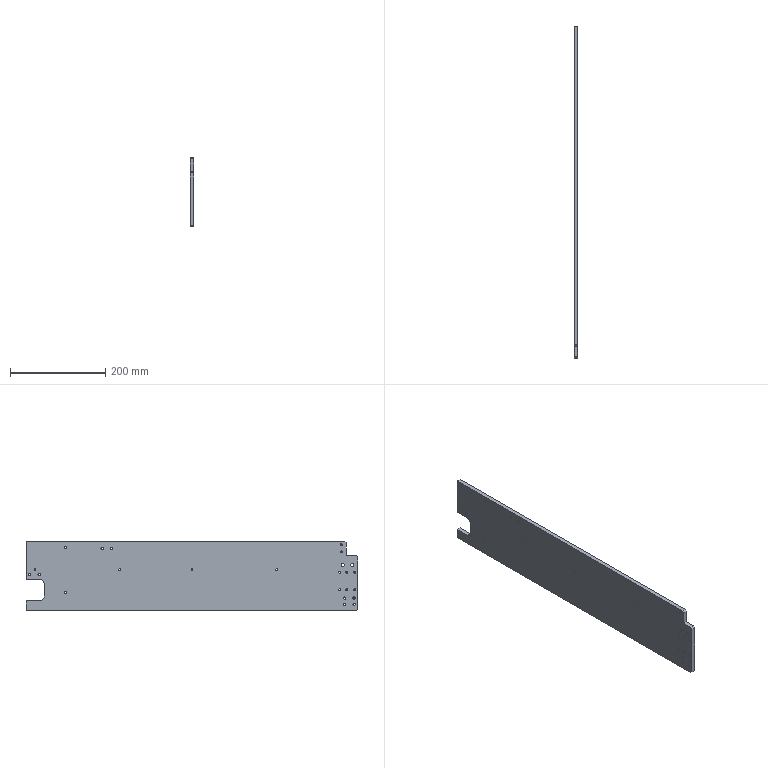Part | NX | features 5003_212_Side plate 2 | 1 solid | 43 faces | box 8 x 698 x 146 mm | volume 792240 mm3 | cylinder 26 | plane 15 | cone 2 | commonest cylinder face diameters 5 x10 4.2 x8 3.3 x4 6.6 x2 20 x2
STEP:
#1=CARTESIAN_POINT('',(-196.775,-63.6,-39.5));
#2=VERTEX_POINT('',#1);
#3=CARTESIAN_POINT('',(-196.775,-63.6,-42.));
#4=DIRECTION('',(1.,0.,0.));
#5=DIRECTION('',(0.,0.,1.));
#6=AXIS2_PLACEMENT_3D('',#3,#4,#5);
#7=CIRCLE('',#6,2.5);
#8=EDGE_CURVE('',#2,#2,#7,.T.);
#9=ORIENTED_EDGE('',*,*,#8,.T.);
#10=EDGE_LOOP('',(#9));
#11=FACE_BOUND('',#10,.T.);
#12=CARTESIAN_POINT('',(-196.775,-83.6,-39.5));
#13=VERTEX_POINT('',#12);
#14=CARTESIAN_POINT('',(-196.775,-83.6,-42.));
#15=DIRECTION('',(1.,0.,0.));
#16=DIRECTION('',(0.,0.,1.));
#17=AXIS2_PLACEMENT_3D('',#14,#15,#16);
#18=CIRCLE('',#17,2.5);
#19=EDGE_CURVE('',#13,#13,#18,.T.);
#20=ORIENTED_EDGE('',*,*,#19,.T.);
#21=EDGE_LOOP('',(#20));
#22=FACE_BOUND('',#21,.T.);
#23=CARTESIAN_POINT('',(-196.775,77.6,-88.15));
#24=VERTEX_POINT('',#23);
#25=CARTESIAN_POINT('',(-196.775,77.6,-86.5));
#26=DIRECTION('',(-1.,0.,0.));
#27=DIRECTION('',(0.,0.,-1.));
#28=AXIS2_PLACEMENT_3D('',#25,#26,#27);
#29=CIRCLE('',#28,1.65);
#30=EDGE_CURVE('',#24,#24,#29,.T.);
#31=ORIENTED_EDGE('',*,*,#30,.F.);
#32=EDGE_LOOP('',(#31));
#33=FACE_BOUND('',#32,.T.);
#34=CARTESIAN_POINT('',(-196.775,-100.2,-88.15));
#35=VERTEX_POINT('',#34);
#36=CARTESIAN_POINT('',(-196.775,-100.2,-86.5));
#37=DIRECTION('',(-1.,0.,0.));
#38=DIRECTION('',(0.,0.,-1.));
#39=AXIS2_PLACEMENT_3D('',#36,#37,#38);
#40=CIRCLE('',#39,1.65);
#41=EDGE_CURVE('',#35,#35,#40,.T.);
#42=ORIENTED_EDGE('',*,*,#41,.F.);
#43=EDGE_LOOP('',(#42));
#44=FACE_BOUND('',#43,.T.);
#45=CARTESIAN_POINT('',(-196.775,-430.4,-88.15));
#46=VERTEX_POINT('',#45);
#47=CARTESIAN_POINT('',(-196.775,-430.4,-86.5));
#48=DIRECTION('',(-1.,0.,0.));
#49=DIRECTION('',(0.,0.,-1.));
#50=AXIS2_PLACEMENT_3D('',#47,#48,#49);
#51=CIRCLE('',#50,1.65);
#52=EDGE_CURVE('',#46,#46,#51,.T.);
#53=ORIENTED_EDGE('',*,*,#52,.F.);
#54=EDGE_LOOP('',(#53));
#55=FACE_BOUND('',#54,.T.);
#56=CARTESIAN_POINT('',(-196.775,88.9,-99.58));
#57=VERTEX_POINT('',#56);
#58=CARTESIAN_POINT('',(-196.775,88.9,-97.08));
#59=DIRECTION('',(-1.,0.,0.));
#60=DIRECTION('',(0.,0.,-1.));
#61=AXIS2_PLACEMENT_3D('',#58,#59,#60);
#62=CIRCLE('',#61,2.5);
#63=EDGE_CURVE('',#57,#57,#62,.T.);
#64=ORIENTED_EDGE('',*,*,#63,.F.);
#65=EDGE_LOOP('',(#64));
#66=FACE_BOUND('',#65,.T.);
#67=CARTESIAN_POINT('',(-196.775,68.9,-99.58));
#68=VERTEX_POINT('',#67);
#69=CARTESIAN_POINT('',(-196.775,68.9,-97.08));
#70=DIRECTION('',(-1.,0.,0.));
#71=DIRECTION('',(0.,0.,-1.));
#72=AXIS2_PLACEMENT_3D('',#69,#70,#71);
#73=CIRCLE('',#72,2.5);
#74=EDGE_CURVE('',#68,#68,#73,.T.);
#75=ORIENTED_EDGE('',*,*,#74,.F.);
#76=EDGE_LOOP('',(#75));
#77=FACE_BOUND('',#76,.T.);
#78=CARTESIAN_POINT('',(-196.775,-573.6,-149.));
#79=VERTEX_POINT('',#78);
#80=CARTESIAN_POINT('',(-196.775,-573.6,-146.5));
#81=DIRECTION('',(-1.,0.,0.));
#82=DIRECTION('',(0.,0.,-1.));
#83=AXIS2_PLACEMENT_3D('',#80,#81,#82);
#84=CIRCLE('',#83,2.5);
#85=EDGE_CURVE('',#79,#79,#84,.T.);
#86=ORIENTED_EDGE('',*,*,#85,.F.);
#87=EDGE_LOOP('',(#86));
#88=FACE_BOUND('',#87,.T.);
#89=CARTESIAN_POINT('',(-196.775,-593.6,-149.));
#90=VERTEX_POINT('',#89);
#91=CARTESIAN_POINT('',(-196.775,-593.6,-146.5));
#92=DIRECTION('',(-1.,0.,0.));
#93=DIRECTION('',(0.,0.,-1.));
#94=AXIS2_PLACEMENT_3D('',#91,#92,#93);
#95=CIRCLE('',#94,2.5);
#96=EDGE_CURVE('',#90,#90,#95,.T.);
#97=ORIENTED_EDGE('',*,*,#96,.F.);
#98=EDGE_LOOP('',(#97));
#99=FACE_BOUND('',#98,.T.);
#100=CARTESIAN_POINT('',(-196.775,-593.6,-162.));
#101=VERTEX_POINT('',#100);
#102=CARTESIAN_POINT('',(-196.775,-593.6,-159.5));
#103=DIRECTION('',(-1.,0.,0.));
#104=DIRECTION('',(0.,0.,-1.));
#105=AXIS2_PLACEMENT_3D('',#102,#103,#104);
#106=CIRCLE('',#105,2.5);
#107=EDGE_CURVE('',#101,#101,#106,.T.);
#108=ORIENTED_EDGE('',*,*,#107,.F.);
#109=EDGE_LOOP('',(#108));
#110=FACE_BOUND('',#109,.T.);
#111=CARTESIAN_POINT('',(-196.775,13.9,-137.));
#112=VERTEX_POINT('',#111);
#113=CARTESIAN_POINT('',(-196.775,13.9,-134.5));
#114=DIRECTION('',(-1.,0.,0.));
#115=DIRECTION('',(0.,0.,-1.));
#116=AXIS2_PLACEMENT_3D('',#113,#114,#115);
#117=CIRCLE('',#116,2.5);
#118=EDGE_CURVE('',#112,#112,#117,.T.);
#119=ORIENTED_EDGE('',*,*,#118,.F.);
#120=EDGE_LOOP('',(#119));
#121=FACE_BOUND('',#120,.T.);
#122=CARTESIAN_POINT('',(-196.775,-566.6,-36.6));
#123=VERTEX_POINT('',#122);
#124=CARTESIAN_POINT('',(-196.775,-566.6,-34.5));
#125=DIRECTION('',(-1.,0.,0.));
#126=DIRECTION('',(0.,0.,-1.));
#127=AXIS2_PLACEMENT_3D('',#124,#125,#126);
#128=CIRCLE('',#127,2.1);
#129=EDGE_CURVE('',#123,#123,#128,.T.);
#130=ORIENTED_EDGE('',*,*,#129,.F.);
#131=EDGE_LOOP('',(#130));
#132=FACE_BOUND('',#131,.T.);
#133=CARTESIAN_POINT('',(-196.775,-566.6,-51.6));
#134=VERTEX_POINT('',#133);
#135=CARTESIAN_POINT('',(-196.775,-566.6,-49.5));
#136=DIRECTION('',(-1.,0.,0.));
#137=DIRECTION('',(0.,0.,-1.));
#138=AXIS2_PLACEMENT_3D('',#135,#136,#137);
#139=CIRCLE('',#138,2.1);
#140=EDGE_CURVE('',#134,#134,#139,.T.);
#141=ORIENTED_EDGE('',*,*,#140,.F.);
#142=EDGE_LOOP('',(#141));
#143=FACE_BOUND('',#142,.T.);
#144=CARTESIAN_POINT('',(-196.775,-563.1,-94.1));
#145=VERTEX_POINT('',#144);
#146=CARTESIAN_POINT('',(-196.775,-563.1,-92.));
#147=DIRECTION('',(-1.,0.,0.));
#148=DIRECTION('',(0.,0.,-1.));
#149=AXIS2_PLACEMENT_3D('',#146,#147,#148);
#150=CIRCLE('',#149,2.1);
#151=EDGE_CURVE('',#145,#145,#150,.T.);
#152=ORIENTED_EDGE('',*,*,#151,.F.);
#153=EDGE_LOOP('',(#152));
#154=FACE_BOUND('',#153,.T.);
#155=CARTESIAN_POINT('',(-196.775,-578.1,-94.1));
#156=VERTEX_POINT('',#155);
#157=CARTESIAN_POINT('',(-196.775,-578.1,-92.));
#158=DIRECTION('',(-1.,0.,0.));
#159=DIRECTION('',(0.,0.,-1.));
#160=AXIS2_PLACEMENT_3D('',#157,#158,#159);
#161=CIRCLE('',#160,2.1);
#162=EDGE_CURVE('',#156,#156,#161,.T.);
#163=ORIENTED_EDGE('',*,*,#162,.F.);
#164=EDGE_LOOP('',(#163));
#165=FACE_BOUND('',#164,.T.);
#166=CARTESIAN_POINT('',(-196.775,-595.1,-94.1));
#167=VERTEX_POINT('',#166);
#168=CARTESIAN_POINT('',(-196.775,-595.1,-92.));
#169=DIRECTION('',(-1.,0.,0.));
#170=DIRECTION('',(0.,0.,-1.));
#171=AXIS2_PLACEMENT_3D('',#168,#169,#170);
#172=CIRCLE('',#171,2.1);
#173=EDGE_CURVE('',#167,#167,#172,.T.);
#174=ORIENTED_EDGE('',*,*,#173,.F.);
#175=EDGE_LOOP('',(#174));
#176=FACE_BOUND('',#175,.T.);
#177=CARTESIAN_POINT('',(-196.775,-595.1,-131.1));
#178=VERTEX_POINT('',#177);
#179=CARTESIAN_POINT('',(-196.775,-595.1,-129.));
#180=DIRECTION('',(-1.,0.,0.));
#181=DIRECTION('',(0.,0.,-1.));
#182=AXIS2_PLACEMENT_3D('',#179,#180,#181);
#183=CIRCLE('',#182,2.1);
#184=EDGE_CURVE('',#178,#178,#183,.T.);
#185=ORIENTED_EDGE('',*,*,#184,.F.);
#186=EDGE_LOOP('',(#185));
#187=FACE_BOUND('',#186,.T.);
#188=CARTESIAN_POINT('',(-196.775,-578.1,-131.1));
#189=VERTEX_POINT('',#188);
#190=CARTESIAN_POINT('',(-196.775,-578.1,-129.));
#191=DIRECTION('',(-1.,0.,0.));
#192=DIRECTION('',(0.,0.,-1.));
#193=AXIS2_PLACEMENT_3D('',#190,#191,#192);
#194=CIRCLE('',#193,2.1);
#195=EDGE_CURVE('',#189,#189,#194,.T.);
#196=ORIENTED_EDGE('',*,*,#195,.F.);
#197=EDGE_LOOP('',(#196));
#198=FACE_BOUND('',#197,.T.);
#199=CARTESIAN_POINT('',(-196.775,-563.1,-131.1));
#200=VERTEX_POINT('',#199);
#201=CARTESIAN_POINT('',(-196.775,-563.1,-129.));
#202=DIRECTION('',(-1.,0.,0.));
#203=DIRECTION('',(0.,0.,-1.));
#204=AXIS2_PLACEMENT_3D('',#201,#202,#203);
#205=CIRCLE('',#204,2.1);
#206=EDGE_CURVE('',#200,#200,#205,.T.);
#207=ORIENTED_EDGE('',*,*,#206,.F.);
#208=EDGE_LOOP('',(#207));
#209=FACE_BOUND('',#208,.T.);
#210=CARTESIAN_POINT('',(-196.775,-569.6,-73.7));
#211=VERTEX_POINT('',#210);
#212=CARTESIAN_POINT('',(-196.775,-569.6,-77.));
#213=DIRECTION('',(1.,0.,0.));
#214=DIRECTION('',(0.,0.,1.));
#215=AXIS2_PLACEMENT_3D('',#212,#213,#214);
#216=CIRCLE('',#215,3.3);
#217=EDGE_CURVE('',#211,#211,#216,.T.);
#218=ORIENTED_EDGE('',*,*,#217,.T.);
#219=EDGE_LOOP('',(#218));
#220=FACE_BOUND('',#219,.T.);
#221=CARTESIAN_POINT('',(-196.775,-589.6,-73.7));
#222=VERTEX_POINT('',#221);
#223=CARTESIAN_POINT('',(-196.775,-589.6,-77.));
#224=DIRECTION('',(1.,0.,0.));
#225=DIRECTION('',(0.,0.,1.));
#226=AXIS2_PLACEMENT_3D('',#223,#224,#225);
#227=CIRCLE('',#226,3.3);
#228=EDGE_CURVE('',#222,#222,#227,.T.);
#229=ORIENTED_EDGE('',*,*,#228,.T.);
#230=EDGE_LOOP('',(#229));
#231=FACE_BOUND('',#230,.T.);
#232=CARTESIAN_POINT('',(-196.775,96.4,-173.));
#233=VERTEX_POINT('',#232);
#234=CARTESIAN_POINT('',(-196.775,-598.6,-173.));
#235=VERTEX_POINT('',#234);
#236=CARTESIAN_POINT('',(-196.775,-601.6,-173.));
#237=DIRECTION('',(0.,-1.,0.));
#238=VECTOR('',#237,1000.);
#239=LINE('',#236,#238);
#240=EDGE_CURVE('',#233,#235,#239,.T.);
#241=ORIENTED_EDGE('',*,*,#240,.T.);
#242=CARTESIAN_POINT('',(-196.775,-601.6,-170.));
#243=VERTEX_POINT('',#242);
#244=CARTESIAN_POINT('',(-196.775,-601.6,-170.));
#245=DIRECTION('',(0.,0.7071,-0.7071));
#246=VECTOR('',#245,1000.);
#247=LINE('',#244,#246);
#248=EDGE_CURVE('',#235,#243,#247,.F.);
#249=ORIENTED_EDGE('',*,*,#248,.T.);
#250=CARTESIAN_POINT('',(-196.775,-601.6,-60.));
#251=VERTEX_POINT('',#250);
#252=CARTESIAN_POINT('',(-196.775,-601.6,-57.));
#253=DIRECTION('',(0.,0.,1.));
#254=VECTOR('',#253,1000.);
#255=LINE('',#252,#254);
#256=EDGE_CURVE('',#243,#251,#255,.T.);
#257=ORIENTED_EDGE('',*,*,#256,.T.);
#258=CARTESIAN_POINT('',(-196.775,-598.6,-57.));
#259=VERTEX_POINT('',#258);
#260=CARTESIAN_POINT('',(-196.775,-598.6,-57.));
#261=DIRECTION('',(0.,-0.7071,-0.7071));
#262=VECTOR('',#261,1000.);
#263=LINE('',#260,#262);
#264=EDGE_CURVE('',#251,#259,#263,.F.);
#265=ORIENTED_EDGE('',*,*,#264,.T.);
#266=CARTESIAN_POINT('',(-196.775,-576.6,-57.));
#267=VERTEX_POINT('',#266);
#268=CARTESIAN_POINT('',(-196.775,-576.6,-57.));
#269=DIRECTION('',(0.,1.,0.));
#270=VECTOR('',#269,1000.);
#271=LINE('',#268,#270);
#272=EDGE_CURVE('',#259,#267,#271,.T.);
#273=ORIENTED_EDGE('',*,*,#272,.T.);
#274=CARTESIAN_POINT('',(-196.775,-576.6,-30.));
#275=VERTEX_POINT('',#274);
#276=CARTESIAN_POINT('',(-196.775,-576.6,-27.));
#277=DIRECTION('',(0.,0.,1.));
#278=VECTOR('',#277,1000.);
#279=LINE('',#276,#278);
#280=EDGE_CURVE('',#267,#275,#279,.T.);
#281=ORIENTED_EDGE('',*,*,#280,.T.);
#282=CARTESIAN_POINT('',(-196.775,-573.6,-27.));
#283=VERTEX_POINT('',#282);
#284=CARTESIAN_POINT('',(-196.775,-573.6,-27.));
#285=DIRECTION('',(0.,-0.7071,-0.7071));
#286=VECTOR('',#285,1000.);
#287=LINE('',#284,#286);
#288=EDGE_CURVE('',#275,#283,#287,.F.);
#289=ORIENTED_EDGE('',*,*,#288,.T.);
#290=CARTESIAN_POINT('',(-196.775,96.4,-27.));
#291=VERTEX_POINT('',#290);
#292=CARTESIAN_POINT('',(-196.775,96.4,-27.));
#293=DIRECTION('',(0.,1.,0.));
#294=VECTOR('',#293,1000.);
#295=LINE('',#292,#294);
#296=EDGE_CURVE('',#283,#291,#295,.T.);
#297=ORIENTED_EDGE('',*,*,#296,.T.);
#298=CARTESIAN_POINT('',(-196.775,96.4,-107.));
#299=VERTEX_POINT('',#298);
#300=CARTESIAN_POINT('',(-196.775,96.4,-107.));
#301=DIRECTION('',(0.,0.,-1.));
#302=VECTOR('',#301,1000.);
#303=LINE('',#300,#302);
#304=EDGE_CURVE('',#291,#299,#303,.T.);
#305=ORIENTED_EDGE('',*,*,#304,.T.);
#306=CARTESIAN_POINT('',(-196.775,68.4,-107.));
#307=VERTEX_POINT('',#306);
#308=CARTESIAN_POINT('',(-196.775,58.4,-107.));
#309=DIRECTION('',(0.,-1.,0.));
#310=VECTOR('',#309,1000.);
#311=LINE('',#308,#310);
#312=EDGE_CURVE('',#299,#307,#311,.T.);
#313=ORIENTED_EDGE('',*,*,#312,.T.);
#314=CARTESIAN_POINT('',(-196.775,58.4,-117.));
#315=VERTEX_POINT('',#314);
#316=CARTESIAN_POINT('',(-196.775,68.4,-117.));
#317=DIRECTION('',(1.,0.,0.));
#318=DIRECTION('',(0.,0.,1.));
#319=AXIS2_PLACEMENT_3D('',#316,#317,#318);
#320=CIRCLE('',#319,10.);
#321=EDGE_CURVE('',#307,#315,#320,.T.);
#322=ORIENTED_EDGE('',*,*,#321,.T.);
#323=CARTESIAN_POINT('',(-196.775,58.4,-142.));
#324=VERTEX_POINT('',#323);
#325=CARTESIAN_POINT('',(-196.775,58.4,-152.));
#326=DIRECTION('',(0.,0.,-1.));
#327=VECTOR('',#326,1000.);
#328=LINE('',#325,#327);
#329=EDGE_CURVE('',#315,#324,#328,.T.);
#330=ORIENTED_EDGE('',*,*,#329,.T.);
#331=CARTESIAN_POINT('',(-196.775,68.4,-152.));
#332=VERTEX_POINT('',#331);
#333=CARTESIAN_POINT('',(-196.775,68.4,-142.));
#334=DIRECTION('',(1.,0.,0.));
#335=DIRECTION('',(0.,0.,1.));
#336=AXIS2_PLACEMENT_3D('',#333,#334,#335);
#337=CIRCLE('',#336,10.);
#338=EDGE_CURVE('',#324,#332,#337,.T.);
#339=ORIENTED_EDGE('',*,*,#338,.T.);
#340=CARTESIAN_POINT('',(-196.775,96.4,-152.));
#341=VERTEX_POINT('',#340);
#342=CARTESIAN_POINT('',(-196.775,96.4,-152.));
#343=DIRECTION('',(0.,1.,0.));
#344=VECTOR('',#343,1000.);
#345=LINE('',#342,#344);
#346=EDGE_CURVE('',#332,#341,#345,.T.);
#347=ORIENTED_EDGE('',*,*,#346,.T.);
#348=CARTESIAN_POINT('',(-196.775,96.4,-173.));
#349=DIRECTION('',(0.,0.,-1.));
#350=VECTOR('',#349,1000.);
#351=LINE('',#348,#350);
#352=EDGE_CURVE('',#341,#233,#351,.T.);
#353=ORIENTED_EDGE('',*,*,#352,.T.);
#354=EDGE_LOOP('',(#241,#249,#257,#265,#273,#281,#289,#297,#305,#313,#322,#330,#339,#347,#353));
#355=FACE_BOUND('',#354,.T.);
#356=CARTESIAN_POINT('',(-196.775,13.9,-42.));
#357=VERTEX_POINT('',#356);
#358=CARTESIAN_POINT('',(-196.775,13.9,-39.5));
#359=DIRECTION('',(-1.,0.,0.));
#360=DIRECTION('',(0.,0.,-1.));
#361=AXIS2_PLACEMENT_3D('',#358,#359,#360);
#362=CIRCLE('',#361,2.5);
#363=EDGE_CURVE('',#357,#357,#362,.T.);
#364=ORIENTED_EDGE('',*,*,#363,.F.);
#365=EDGE_LOOP('',(#364));
#366=FACE_BOUND('',#365,.T.);
#367=CARTESIAN_POINT('',(-196.775,-573.6,-162.));
#368=VERTEX_POINT('',#367);
#369=CARTESIAN_POINT('',(-196.775,-573.6,-159.5));
#370=DIRECTION('',(-1.,0.,0.));
#371=DIRECTION('',(0.,0.,-1.));
#372=AXIS2_PLACEMENT_3D('',#369,#370,#371);
#373=CIRCLE('',#372,2.5);
#374=EDGE_CURVE('',#368,#368,#373,.T.);
#375=ORIENTED_EDGE('',*,*,#374,.F.);
#376=EDGE_LOOP('',(#375));
#377=FACE_BOUND('',#376,.T.);
#378=CARTESIAN_POINT('',(-196.775,-252.6,-88.15));
#379=VERTEX_POINT('',#378);
#380=CARTESIAN_POINT('',(-196.775,-252.6,-86.5));
#381=DIRECTION('',(-1.,0.,0.));
#382=DIRECTION('',(0.,0.,-1.));
#383=AXIS2_PLACEMENT_3D('',#380,#381,#382);
#384=CIRCLE('',#383,1.65);
#385=EDGE_CURVE('',#379,#379,#384,.T.);
#386=ORIENTED_EDGE('',*,*,#385,.F.);
#387=EDGE_LOOP('',(#386));
#388=FACE_BOUND('',#387,.T.);
#389=CARTESIAN_POINT('',(-196.775,96.4,-27.));
#390=DIRECTION('',(1.,0.,0.));
#391=DIRECTION('',(0.,0.,1.));
#392=AXIS2_PLACEMENT_3D('',#389,#390,#391);
#393=PLANE('',#392);
#394=ADVANCED_FACE('',(#11,#22,#33,#44,#55,#66,#77,#88,#99,#110,#121,#132,#143,#154,#165,#176,#187,#198,#209,#220,#231,#355,#366,#377,#388),#393,.F.);
#395=CARTESIAN_POINT('',(-188.775,96.4,-27.));
#396=VERTEX_POINT('',#395);
#397=CARTESIAN_POINT('',(-188.775,96.4,-107.));
#398=VERTEX_POINT('',#397);
#399=CARTESIAN_POINT('',(-188.775,96.4,-107.));
#400=DIRECTION('',(0.,0.,-1.));
#401=VECTOR('',#400,1000.);
#402=LINE('',#399,#401);
#403=EDGE_CURVE('',#396,#398,#402,.T.);
#404=ORIENTED_EDGE('',*,*,#403,.T.);
#405=CARTESIAN_POINT('',(-196.775,96.4,-107.));
#406=DIRECTION('',(1.,0.,0.));
#407=VECTOR('',#406,1000.);
#408=LINE('',#405,#407);
#409=EDGE_CURVE('',#299,#398,#408,.T.);
#410=ORIENTED_EDGE('',*,*,#409,.F.);
#411=ORIENTED_EDGE('',*,*,#304,.F.);
#412=CARTESIAN_POINT('',(-196.775,96.4,-27.));
#413=DIRECTION('',(1.,0.,0.));
#414=VECTOR('',#413,1000.);
#415=LINE('',#412,#414);
#416=EDGE_CURVE('',#291,#396,#415,.T.);
#417=ORIENTED_EDGE('',*,*,#416,.T.);
#418=EDGE_LOOP('',(#404,#410,#411,#417));
#419=FACE_BOUND('',#418,.T.);
#420=CARTESIAN_POINT('',(-196.775,96.4,-107.));
#421=DIRECTION('',(0.,-1.,0.));
#422=DIRECTION('',(0.,0.,1.));
#423=AXIS2_PLACEMENT_3D('',#420,#421,#422);
#424=PLANE('',#423);
#425=ADVANCED_FACE('',(#419),#424,.F.);
#426=CARTESIAN_POINT('',(-188.775,68.4,-107.));
#427=VERTEX_POINT('',#426);
#428=CARTESIAN_POINT('',(-188.775,58.4,-107.));
#429=DIRECTION('',(0.,-1.,0.));
#430=VECTOR('',#429,1000.);
#431=LINE('',#428,#430);
#432=EDGE_CURVE('',#398,#427,#431,.T.);
#433=ORIENTED_EDGE('',*,*,#432,.T.);
#434=CARTESIAN_POINT('',(-196.775,68.4,-107.));
#435=DIRECTION('',(1.,0.,0.));
#436=VECTOR('',#435,1000.);
#437=LINE('',#434,#436);
#438=EDGE_CURVE('',#427,#307,#437,.F.);
#439=ORIENTED_EDGE('',*,*,#438,.T.);
#440=ORIENTED_EDGE('',*,*,#312,.F.);
#441=ORIENTED_EDGE('',*,*,#409,.T.);
#442=EDGE_LOOP('',(#433,#439,#440,#441));
#443=FACE_BOUND('',#442,.T.);
#444=CARTESIAN_POINT('',(-196.775,58.4,-107.));
#445=DIRECTION('',(0.,0.,1.));
#446=DIRECTION('',(0.,1.,0.));
#447=AXIS2_PLACEMENT_3D('',#444,#445,#446);
#448=PLANE('',#447);
#449=ADVANCED_FACE('',(#443),#448,.F.);
#450=CARTESIAN_POINT('',(-188.775,58.4,-117.));
#451=VERTEX_POINT('',#450);
#452=CARTESIAN_POINT('',(-188.775,58.4,-142.));
#453=VERTEX_POINT('',#452);
#454=CARTESIAN_POINT('',(-188.775,58.4,-152.));
#455=DIRECTION('',(0.,0.,-1.));
#456=VECTOR('',#455,1000.);
#457=LINE('',#454,#456);
#458=EDGE_CURVE('',#451,#453,#457,.T.);
#459=ORIENTED_EDGE('',*,*,#458,.T.);
#460=CARTESIAN_POINT('',(-196.775,58.4,-142.));
#461=DIRECTION('',(1.,0.,0.));
#462=VECTOR('',#461,1000.);
#463=LINE('',#460,#462);
#464=EDGE_CURVE('',#453,#324,#463,.F.);
#465=ORIENTED_EDGE('',*,*,#464,.T.);
#466=ORIENTED_EDGE('',*,*,#329,.F.);
#467=CARTESIAN_POINT('',(-188.775,58.4,-117.));
#468=DIRECTION('',(1.,0.,0.));
#469=VECTOR('',#468,1000.);
#470=LINE('',#467,#469);
#471=EDGE_CURVE('',#315,#451,#470,.T.);
#472=ORIENTED_EDGE('',*,*,#471,.T.);
#473=EDGE_LOOP('',(#459,#465,#466,#472));
#474=FACE_BOUND('',#473,.T.);
#475=CARTESIAN_POINT('',(-196.775,58.4,-152.));
#476=DIRECTION('',(0.,-1.,0.));
#477=DIRECTION('',(0.,0.,1.));
#478=AXIS2_PLACEMENT_3D('',#475,#476,#477);
#479=PLANE('',#478);
#480=ADVANCED_FACE('',(#474),#479,.F.);
#481=ORIENTED_EDGE('',*,*,#346,.F.);
#482=CARTESIAN_POINT('',(-188.775,68.4,-152.));
#483=VERTEX_POINT('',#482);
#484=CARTESIAN_POINT('',(-188.775,68.4,-152.));
#485=DIRECTION('',(1.,0.,0.));
#486=VECTOR('',#485,1000.);
#487=LINE('',#484,#486);
#488=EDGE_CURVE('',#332,#483,#487,.T.);
#489=ORIENTED_EDGE('',*,*,#488,.T.);
#490=CARTESIAN_POINT('',(-188.775,96.4,-152.));
#491=VERTEX_POINT('',#490);
#492=CARTESIAN_POINT('',(-188.775,96.4,-152.));
#493=DIRECTION('',(0.,1.,0.));
#494=VECTOR('',#493,1000.);
#495=LINE('',#492,#494);
#496=EDGE_CURVE('',#483,#491,#495,.T.);
#497=ORIENTED_EDGE('',*,*,#496,.T.);
#498=CARTESIAN_POINT('',(-196.775,96.4,-152.));
#499=DIRECTION('',(1.,0.,0.));
#500=VECTOR('',#499,1000.);
#501=LINE('',#498,#500);
#502=EDGE_CURVE('',#341,#491,#501,.T.);
#503=ORIENTED_EDGE('',*,*,#502,.F.);
#504=EDGE_LOOP('',(#481,#489,#497,#503));
#505=FACE_BOUND('',#504,.T.);
#506=CARTESIAN_POINT('',(-196.775,96.4,-152.));
#507=DIRECTION('',(0.,0.,-1.));
#508=DIRECTION('',(0.,-1.,0.));
#509=AXIS2_PLACEMENT_3D('',#506,#507,#508);
#510=PLANE('',#509);
#511=ADVANCED_FACE('',(#505),#510,.F.);
#512=CARTESIAN_POINT('',(-188.775,96.4,-173.));
#513=VERTEX_POINT('',#512);
#514=CARTESIAN_POINT('',(-188.775,96.4,-173.));
#515=DIRECTION('',(0.,0.,-1.));
#516=VECTOR('',#515,1000.);
#517=LINE('',#514,#516);
#518=EDGE_CURVE('',#491,#513,#517,.T.);
#519=ORIENTED_EDGE('',*,*,#518,.T.);
#520=CARTESIAN_POINT('',(-196.775,96.4,-173.));
#521=DIRECTION('',(1.,0.,0.));
#522=VECTOR('',#521,1000.);
#523=LINE('',#520,#522);
#524=EDGE_CURVE('',#233,#513,#523,.T.);
#525=ORIENTED_EDGE('',*,*,#524,.F.);
#526=ORIENTED_EDGE('',*,*,#352,.F.);
#527=ORIENTED_EDGE('',*,*,#502,.T.);
#528=EDGE_LOOP('',(#519,#525,#526,#527));
#529=FACE_BOUND('',#528,.T.);
#530=CARTESIAN_POINT('',(-196.775,96.4,-173.));
#531=DIRECTION('',(0.,-1.,0.));
#532=DIRECTION('',(0.,0.,1.));
#533=AXIS2_PLACEMENT_3D('',#530,#531,#532);
#534=PLANE('',#533);
#535=ADVANCED_FACE('',(#529),#534,.F.);
#536=CARTESIAN_POINT('',(-188.775,-598.6,-173.));
#537=VERTEX_POINT('',#536);
#538=CARTESIAN_POINT('',(-188.775,-601.6,-173.));
#539=DIRECTION('',(0.,-1.,0.));
#540=VECTOR('',#539,1000.);
#541=LINE('',#538,#540);
#542=EDGE_CURVE('',#513,#537,#541,.T.);
#543=ORIENTED_EDGE('',*,*,#542,.T.);
#544=CARTESIAN_POINT('',(-196.775,-598.6,-173.));
#545=DIRECTION('',(-1.,0.,0.));
#546=VECTOR('',#545,1000.);
#547=LINE('',#544,#546);
#548=EDGE_CURVE('',#537,#235,#547,.T.);
#549=ORIENTED_EDGE('',*,*,#548,.T.);
#550=ORIENTED_EDGE('',*,*,#240,.F.);
#551=ORIENTED_EDGE('',*,*,#524,.T.);
#552=EDGE_LOOP('',(#543,#549,#550,#551));
#553=FACE_BOUND('',#552,.T.);
#554=CARTESIAN_POINT('',(-196.775,-601.6,-173.));
#555=DIRECTION('',(0.,0.,1.));
#556=DIRECTION('',(0.,1.,0.));
#557=AXIS2_PLACEMENT_3D('',#554,#555,#556);
#558=PLANE('',#557);
#559=ADVANCED_FACE('',(#553),#558,.F.);
#560=ORIENTED_EDGE('',*,*,#256,.F.);
#561=CARTESIAN_POINT('',(-188.775,-601.6,-170.));
#562=VERTEX_POINT('',#561);
#563=CARTESIAN_POINT('',(-196.775,-601.6,-170.));
#564=DIRECTION('',(1.,0.,0.));
#565=VECTOR('',#564,1000.);
#566=LINE('',#563,#565);
#567=EDGE_CURVE('',#243,#562,#566,.T.);
#568=ORIENTED_EDGE('',*,*,#567,.T.);
#569=CARTESIAN_POINT('',(-188.775,-601.6,-60.));
#570=VERTEX_POINT('',#569);
#571=CARTESIAN_POINT('',(-188.775,-601.6,-57.));
#572=DIRECTION('',(0.,0.,1.));
#573=VECTOR('',#572,1000.);
#574=LINE('',#571,#573);
#575=EDGE_CURVE('',#562,#570,#574,.T.);
#576=ORIENTED_EDGE('',*,*,#575,.T.);
#577=CARTESIAN_POINT('',(-196.775,-601.6,-60.));
#578=DIRECTION('',(-1.,0.,0.));
#579=VECTOR('',#578,1000.);
#580=LINE('',#577,#579);
#581=EDGE_CURVE('',#570,#251,#580,.T.);
#582=ORIENTED_EDGE('',*,*,#581,.T.);
#583=EDGE_LOOP('',(#560,#568,#576,#582));
#584=FACE_BOUND('',#583,.T.);
#585=CARTESIAN_POINT('',(-196.775,-601.6,-57.));
#586=DIRECTION('',(0.,1.,0.));
#587=DIRECTION('',(0.,0.,-1.));
#588=AXIS2_PLACEMENT_3D('',#585,#586,#587);
#589=PLANE('',#588);
#590=ADVANCED_FACE('',(#584),#589,.F.);
#591=ORIENTED_EDGE('',*,*,#272,.F.);
#592=CARTESIAN_POINT('',(-188.775,-598.6,-57.));
#593=VERTEX_POINT('',#592);
#594=CARTESIAN_POINT('',(-196.775,-598.6,-57.));
#595=DIRECTION('',(1.,0.,0.));
#596=VECTOR('',#595,1000.);
#597=LINE('',#594,#596);
#598=EDGE_CURVE('',#259,#593,#597,.T.);
#599=ORIENTED_EDGE('',*,*,#598,.T.);
#600=CARTESIAN_POINT('',(-188.775,-576.6,-57.));
#601=VERTEX_POINT('',#600);
#602=CARTESIAN_POINT('',(-188.775,-576.6,-57.));
#603=DIRECTION('',(0.,1.,0.));
#604=VECTOR('',#603,1000.);
#605=LINE('',#602,#604);
#606=EDGE_CURVE('',#593,#601,#605,.T.);
#607=ORIENTED_EDGE('',*,*,#606,.T.);
#608=CARTESIAN_POINT('',(-196.775,-576.6,-57.));
#609=DIRECTION('',(1.,0.,0.));
#610=VECTOR('',#609,1000.);
#611=LINE('',#608,#610);
#612=EDGE_CURVE('',#267,#601,#611,.T.);
#613=ORIENTED_EDGE('',*,*,#612,.F.);
#614=EDGE_LOOP('',(#591,#599,#607,#613));
#615=FACE_BOUND('',#614,.T.);
#616=CARTESIAN_POINT('',(-196.775,-576.6,-57.));
#617=DIRECTION('',(0.,0.,-1.));
#618=DIRECTION('',(0.,-1.,0.));
#619=AXIS2_PLACEMENT_3D('',#616,#617,#618);
#620=PLANE('',#619);
#621=ADVANCED_FACE('',(#615),#620,.F.);
#622=CARTESIAN_POINT('',(-188.775,-576.6,-30.));
#623=VERTEX_POINT('',#622);
#624=CARTESIAN_POINT('',(-188.775,-576.6,-27.));
#625=DIRECTION('',(0.,0.,1.));
#626=VECTOR('',#625,1000.);
#627=LINE('',#624,#626);
#628=EDGE_CURVE('',#601,#623,#627,.T.);
#629=ORIENTED_EDGE('',*,*,#628,.T.);
#630=CARTESIAN_POINT('',(-196.775,-576.6,-30.));
#631=DIRECTION('',(-1.,0.,0.));
#632=VECTOR('',#631,1000.);
#633=LINE('',#630,#632);
#634=EDGE_CURVE('',#623,#275,#633,.T.);
#635=ORIENTED_EDGE('',*,*,#634,.T.);
#636=ORIENTED_EDGE('',*,*,#280,.F.);
#637=ORIENTED_EDGE('',*,*,#612,.T.);
#638=EDGE_LOOP('',(#629,#635,#636,#637));
#639=FACE_BOUND('',#638,.T.);
#640=CARTESIAN_POINT('',(-196.775,-576.6,-27.));
#641=DIRECTION('',(0.,1.,0.));
#642=DIRECTION('',(0.,0.,-1.));
#643=AXIS2_PLACEMENT_3D('',#640,#641,#642);
#644=PLANE('',#643);
#645=ADVANCED_FACE('',(#639),#644,.F.);
#646=ORIENTED_EDGE('',*,*,#296,.F.);
#647=CARTESIAN_POINT('',(-188.775,-573.6,-27.));
#648=VERTEX_POINT('',#647);
#649=CARTESIAN_POINT('',(-196.775,-573.6,-27.));
#650=DIRECTION('',(1.,0.,0.));
#651=VECTOR('',#650,1000.);
#652=LINE('',#649,#651);
#653=EDGE_CURVE('',#283,#648,#652,.T.);
#654=ORIENTED_EDGE('',*,*,#653,.T.);
#655=CARTESIAN_POINT('',(-188.775,96.4,-27.));
#656=DIRECTION('',(0.,1.,0.));
#657=VECTOR('',#656,1000.);
#658=LINE('',#655,#657);
#659=EDGE_CURVE('',#648,#396,#658,.T.);
#660=ORIENTED_EDGE('',*,*,#659,.T.);
#661=ORIENTED_EDGE('',*,*,#416,.F.);
#662=EDGE_LOOP('',(#646,#654,#660,#661));
#663=FACE_BOUND('',#662,.T.);
#664=CARTESIAN_POINT('',(-196.775,96.4,-27.));
#665=DIRECTION('',(0.,0.,-1.));
#666=DIRECTION('',(0.,-1.,0.));
#667=AXIS2_PLACEMENT_3D('',#664,#665,#666);
#668=PLANE('',#667);
#669=ADVANCED_FACE('',(#663),#668,.F.);
#670=CARTESIAN_POINT('',(-188.775,-63.6,-39.5));
#671=VERTEX_POINT('',#670);
#672=CARTESIAN_POINT('',(-188.775,-63.6,-42.));
#673=DIRECTION('',(1.,0.,0.));
#674=DIRECTION('',(0.,0.,1.));
#675=AXIS2_PLACEMENT_3D('',#672,#673,#674);
#676=CIRCLE('',#675,2.5);
#677=EDGE_CURVE('',#671,#671,#676,.T.);
#678=ORIENTED_EDGE('',*,*,#677,.F.);
#679=EDGE_LOOP('',(#678));
#680=FACE_BOUND('',#679,.T.);
#681=CARTESIAN_POINT('',(-188.775,-83.6,-39.5));
#682=VERTEX_POINT('',#681);
#683=CARTESIAN_POINT('',(-188.775,-83.6,-42.));
#684=DIRECTION('',(1.,0.,0.));
#685=DIRECTION('',(0.,0.,1.));
#686=AXIS2_PLACEMENT_3D('',#683,#684,#685);
#687=CIRCLE('',#686,2.5);
#688=EDGE_CURVE('',#682,#682,#687,.T.);
#689=ORIENTED_EDGE('',*,*,#688,.F.);
#690=EDGE_LOOP('',(#689));
#691=FACE_BOUND('',#690,.T.);
#692=CARTESIAN_POINT('',(-188.775,77.6,-84.85));
#693=VERTEX_POINT('',#692);
#694=CARTESIAN_POINT('',(-188.775,77.6,-86.5));
#695=DIRECTION('',(1.,0.,0.));
#696=DIRECTION('',(0.,0.,1.));
#697=AXIS2_PLACEMENT_3D('',#694,#695,#696);
#698=CIRCLE('',#697,1.65);
#699=EDGE_CURVE('',#693,#693,#698,.T.);
#700=ORIENTED_EDGE('',*,*,#699,.F.);
#701=EDGE_LOOP('',(#700));
#702=FACE_BOUND('',#701,.T.);
#703=CARTESIAN_POINT('',(-188.775,-100.2,-84.85));
#704=VERTEX_POINT('',#703);
#705=CARTESIAN_POINT('',(-188.775,-100.2,-86.5));
#706=DIRECTION('',(1.,0.,0.));
#707=DIRECTION('',(0.,0.,1.));
#708=AXIS2_PLACEMENT_3D('',#705,#706,#707);
#709=CIRCLE('',#708,1.65);
#710=EDGE_CURVE('',#704,#704,#709,.T.);
#711=ORIENTED_EDGE('',*,*,#710,.F.);
#712=EDGE_LOOP('',(#711));
#713=FACE_BOUND('',#712,.T.);
#714=CARTESIAN_POINT('',(-188.775,-252.6,-84.85));
#715=VERTEX_POINT('',#714);
#716=CARTESIAN_POINT('',(-188.775,-252.6,-86.5));
#717=DIRECTION('',(1.,0.,0.));
#718=DIRECTION('',(0.,0.,1.));
#719=AXIS2_PLACEMENT_3D('',#716,#717,#718);
#720=CIRCLE('',#719,1.65);
#721=EDGE_CURVE('',#715,#715,#720,.T.);
#722=ORIENTED_EDGE('',*,*,#721,.F.);
#723=EDGE_LOOP('',(#722));
#724=FACE_BOUND('',#723,.T.);
#725=CARTESIAN_POINT('',(-188.775,-430.4,-84.85));
#726=VERTEX_POINT('',#725);
#727=CARTESIAN_POINT('',(-188.775,-430.4,-86.5));
#728=DIRECTION('',(1.,0.,0.));
#729=DIRECTION('',(0.,0.,1.));
#730=AXIS2_PLACEMENT_3D('',#727,#728,#729);
#731=CIRCLE('',#730,1.65);
#732=EDGE_CURVE('',#726,#726,#731,.T.);
#733=ORIENTED_EDGE('',*,*,#732,.F.);
#734=EDGE_LOOP('',(#733));
#735=FACE_BOUND('',#734,.T.);
#736=CARTESIAN_POINT('',(-188.775,88.9,-94.58));
#737=VERTEX_POINT('',#736);
#738=CARTESIAN_POINT('',(-188.775,88.9,-97.08));
#739=DIRECTION('',(1.,0.,0.));
#740=DIRECTION('',(0.,0.,1.));
#741=AXIS2_PLACEMENT_3D('',#738,#739,#740);
#742=CIRCLE('',#741,2.5);
#743=EDGE_CURVE('',#737,#737,#742,.T.);
#744=ORIENTED_EDGE('',*,*,#743,.F.);
#745=EDGE_LOOP('',(#744));
#746=FACE_BOUND('',#745,.T.);
#747=CARTESIAN_POINT('',(-188.775,68.9,-94.58));
#748=VERTEX_POINT('',#747);
#749=CARTESIAN_POINT('',(-188.775,68.9,-97.08));
#750=DIRECTION('',(1.,0.,0.));
#751=DIRECTION('',(0.,0.,1.));
#752=AXIS2_PLACEMENT_3D('',#749,#750,#751);
#753=CIRCLE('',#752,2.5);
#754=EDGE_CURVE('',#748,#748,#753,.T.);
#755=ORIENTED_EDGE('',*,*,#754,.F.);
#756=EDGE_LOOP('',(#755));
#757=FACE_BOUND('',#756,.T.);
#758=CARTESIAN_POINT('',(-188.775,-573.6,-144.));
#759=VERTEX_POINT('',#758);
#760=CARTESIAN_POINT('',(-188.775,-573.6,-146.5));
#761=DIRECTION('',(1.,0.,0.));
#762=DIRECTION('',(0.,0.,1.));
#763=AXIS2_PLACEMENT_3D('',#760,#761,#762);
#764=CIRCLE('',#763,2.5);
#765=EDGE_CURVE('',#759,#759,#764,.T.);
#766=ORIENTED_EDGE('',*,*,#765,.F.);
#767=EDGE_LOOP('',(#766));
#768=FACE_BOUND('',#767,.T.);
#769=CARTESIAN_POINT('',(-188.775,-593.6,-144.));
#770=VERTEX_POINT('',#769);
#771=CARTESIAN_POINT('',(-188.775,-593.6,-146.5));
#772=DIRECTION('',(1.,0.,0.));
#773=DIRECTION('',(0.,0.,1.));
#774=AXIS2_PLACEMENT_3D('',#771,#772,#773);
#775=CIRCLE('',#774,2.5);
#776=EDGE_CURVE('',#770,#770,#775,.T.);
#777=ORIENTED_EDGE('',*,*,#776,.F.);
#778=EDGE_LOOP('',(#777));
#779=FACE_BOUND('',#778,.T.);
#780=CARTESIAN_POINT('',(-188.775,-573.6,-157.));
#781=VERTEX_POINT('',#780);
#782=CARTESIAN_POINT('',(-188.775,-573.6,-159.5));
#783=DIRECTION('',(1.,0.,0.));
#784=DIRECTION('',(0.,0.,1.));
#785=AXIS2_PLACEMENT_3D('',#782,#783,#784);
#786=CIRCLE('',#785,2.5);
#787=EDGE_CURVE('',#781,#781,#786,.T.);
#788=ORIENTED_EDGE('',*,*,#787,.F.);
#789=EDGE_LOOP('',(#788));
#790=FACE_BOUND('',#789,.T.);
#791=CARTESIAN_POINT('',(-188.775,-593.6,-157.));
#792=VERTEX_POINT('',#791);
#793=CARTESIAN_POINT('',(-188.775,-593.6,-159.5));
#794=DIRECTION('',(1.,0.,0.));
#795=DIRECTION('',(0.,0.,1.));
#796=AXIS2_PLACEMENT_3D('',#793,#794,#795);
#797=CIRCLE('',#796,2.5);
#798=EDGE_CURVE('',#792,#792,#797,.T.);
#799=ORIENTED_EDGE('',*,*,#798,.F.);
#800=EDGE_LOOP('',(#799));
#801=FACE_BOUND('',#800,.T.);
#802=CARTESIAN_POINT('',(-188.775,13.9,-37.));
#803=VERTEX_POINT('',#802);
#804=CARTESIAN_POINT('',(-188.775,13.9,-39.5));
#805=DIRECTION('',(1.,0.,0.));
#806=DIRECTION('',(0.,0.,1.));
#807=AXIS2_PLACEMENT_3D('',#804,#805,#806);
#808=CIRCLE('',#807,2.5);
#809=EDGE_CURVE('',#803,#803,#808,.T.);
#810=ORIENTED_EDGE('',*,*,#809,.F.);
#811=EDGE_LOOP('',(#810));
#812=FACE_BOUND('',#811,.T.);
#813=CARTESIAN_POINT('',(-188.775,13.9,-132.));
#814=VERTEX_POINT('',#813);
#815=CARTESIAN_POINT('',(-188.775,13.9,-134.5));
#816=DIRECTION('',(1.,0.,0.));
#817=DIRECTION('',(0.,0.,1.));
#818=AXIS2_PLACEMENT_3D('',#815,#816,#817);
#819=CIRCLE('',#818,2.5);
#820=EDGE_CURVE('',#814,#814,#819,.T.);
#821=ORIENTED_EDGE('',*,*,#820,.F.);
#822=EDGE_LOOP('',(#821));
#823=FACE_BOUND('',#822,.T.);
#824=CARTESIAN_POINT('',(-188.775,-566.6,-32.4));
#825=VERTEX_POINT('',#824);
#826=CARTESIAN_POINT('',(-188.775,-566.6,-34.5));
#827=DIRECTION('',(1.,0.,0.));
#828=DIRECTION('',(0.,0.,1.));
#829=AXIS2_PLACEMENT_3D('',#826,#827,#828);
#830=CIRCLE('',#829,2.1);
#831=EDGE_CURVE('',#825,#825,#830,.T.);
#832=ORIENTED_EDGE('',*,*,#831,.F.);
#833=EDGE_LOOP('',(#832));
#834=FACE_BOUND('',#833,.T.);
#835=CARTESIAN_POINT('',(-188.775,-566.6,-47.4));
#836=VERTEX_POINT('',#835);
#837=CARTESIAN_POINT('',(-188.775,-566.6,-49.5));
#838=DIRECTION('',(1.,0.,0.));
#839=DIRECTION('',(0.,0.,1.));
#840=AXIS2_PLACEMENT_3D('',#837,#838,#839);
#841=CIRCLE('',#840,2.1);
#842=EDGE_CURVE('',#836,#836,#841,.T.);
#843=ORIENTED_EDGE('',*,*,#842,.F.);
#844=EDGE_LOOP('',(#843));
#845=FACE_BOUND('',#844,.T.);
#846=CARTESIAN_POINT('',(-188.775,-563.1,-89.9));
#847=VERTEX_POINT('',#846);
#848=CARTESIAN_POINT('',(-188.775,-563.1,-92.));
#849=DIRECTION('',(1.,0.,0.));
#850=DIRECTION('',(0.,0.,1.));
#851=AXIS2_PLACEMENT_3D('',#848,#849,#850);
#852=CIRCLE('',#851,2.1);
#853=EDGE_CURVE('',#847,#847,#852,.T.);
#854=ORIENTED_EDGE('',*,*,#853,.F.);
#855=EDGE_LOOP('',(#854));
#856=FACE_BOUND('',#855,.T.);
#857=CARTESIAN_POINT('',(-188.775,-578.1,-89.9));
#858=VERTEX_POINT('',#857);
#859=CARTESIAN_POINT('',(-188.775,-578.1,-92.));
#860=DIRECTION('',(1.,0.,0.));
#861=DIRECTION('',(0.,0.,1.));
#862=AXIS2_PLACEMENT_3D('',#859,#860,#861);
#863=CIRCLE('',#862,2.1);
#864=EDGE_CURVE('',#858,#858,#863,.T.);
#865=ORIENTED_EDGE('',*,*,#864,.F.);
#866=EDGE_LOOP('',(#865));
#867=FACE_BOUND('',#866,.T.);
#868=CARTESIAN_POINT('',(-188.775,-595.1,-89.9));
#869=VERTEX_POINT('',#868);
#870=CARTESIAN_POINT('',(-188.775,-595.1,-92.));
#871=DIRECTION('',(1.,0.,0.));
#872=DIRECTION('',(0.,0.,1.));
#873=AXIS2_PLACEMENT_3D('',#870,#871,#872);
#874=CIRCLE('',#873,2.1);
#875=EDGE_CURVE('',#869,#869,#874,.T.);
#876=ORIENTED_EDGE('',*,*,#875,.F.);
#877=EDGE_LOOP('',(#876));
#878=FACE_BOUND('',#877,.T.);
#879=CARTESIAN_POINT('',(-188.775,-595.1,-126.9));
#880=VERTEX_POINT('',#879);
#881=CARTESIAN_POINT('',(-188.775,-595.1,-129.));
#882=DIRECTION('',(1.,0.,0.));
#883=DIRECTION('',(0.,0.,1.));
#884=AXIS2_PLACEMENT_3D('',#881,#882,#883);
#885=CIRCLE('',#884,2.1);
#886=EDGE_CURVE('',#880,#880,#885,.T.);
#887=ORIENTED_EDGE('',*,*,#886,.F.);
#888=EDGE_LOOP('',(#887));
#889=FACE_BOUND('',#888,.T.);
#890=CARTESIAN_POINT('',(-188.775,-578.1,-126.9));
#891=VERTEX_POINT('',#890);
#892=CARTESIAN_POINT('',(-188.775,-578.1,-129.));
#893=DIRECTION('',(1.,0.,0.));
#894=DIRECTION('',(0.,0.,1.));
#895=AXIS2_PLACEMENT_3D('',#892,#893,#894);
#896=CIRCLE('',#895,2.1);
#897=EDGE_CURVE('',#891,#891,#896,.T.);
#898=ORIENTED_EDGE('',*,*,#897,.F.);
#899=EDGE_LOOP('',(#898));
#900=FACE_BOUND('',#899,.T.);
#901=CARTESIAN_POINT('',(-188.775,-563.1,-126.9));
#902=VERTEX_POINT('',#901);
#903=CARTESIAN_POINT('',(-188.775,-563.1,-129.));
#904=DIRECTION('',(1.,0.,0.));
#905=DIRECTION('',(0.,0.,1.));
#906=AXIS2_PLACEMENT_3D('',#903,#904,#905);
#907=CIRCLE('',#906,2.1);
#908=EDGE_CURVE('',#902,#902,#907,.T.);
#909=ORIENTED_EDGE('',*,*,#908,.F.);
#910=EDGE_LOOP('',(#909));
#911=FACE_BOUND('',#910,.T.);
#912=CARTESIAN_POINT('',(-188.775,-569.6,-70.4));
#913=VERTEX_POINT('',#912);
#914=CARTESIAN_POINT('',(-188.775,-569.6,-77.));
#915=DIRECTION('',(1.,0.,0.));
#916=DIRECTION('',(0.,0.,1.));
#917=AXIS2_PLACEMENT_3D('',#914,#915,#916);
#918=CIRCLE('',#917,6.6);
#919=EDGE_CURVE('',#913,#913,#918,.T.);
#920=ORIENTED_EDGE('',*,*,#919,.F.);
#921=EDGE_LOOP('',(#920));
#922=FACE_BOUND('',#921,.T.);
#923=CARTESIAN_POINT('',(-188.775,-589.6,-70.4));
#924=VERTEX_POINT('',#923);
#925=CARTESIAN_POINT('',(-188.775,-589.6,-77.));
#926=DIRECTION('',(1.,0.,0.));
#927=DIRECTION('',(0.,0.,1.));
#928=AXIS2_PLACEMENT_3D('',#925,#926,#927);
#929=CIRCLE('',#928,6.6);
#930=EDGE_CURVE('',#924,#924,#929,.T.);
#931=ORIENTED_EDGE('',*,*,#930,.F.);
#932=EDGE_LOOP('',(#931));
#933=FACE_BOUND('',#932,.T.);
#934=ORIENTED_EDGE('',*,*,#575,.F.);
#935=CARTESIAN_POINT('',(-188.775,-324.1,-447.5));
#936=DIRECTION('',(0.,-0.7071,0.7071));
#937=VECTOR('',#936,1000.);
#938=LINE('',#935,#937);
#939=EDGE_CURVE('',#562,#537,#938,.F.);
#940=ORIENTED_EDGE('',*,*,#939,.T.);
#941=ORIENTED_EDGE('',*,*,#542,.F.);
#942=ORIENTED_EDGE('',*,*,#518,.F.);
#943=ORIENTED_EDGE('',*,*,#496,.F.);
#944=CARTESIAN_POINT('',(-188.775,68.4,-142.));
#945=DIRECTION('',(1.,0.,0.));
#946=DIRECTION('',(0.,0.,1.));
#947=AXIS2_PLACEMENT_3D('',#944,#945,#946);
#948=CIRCLE('',#947,10.);
#949=EDGE_CURVE('',#483,#453,#948,.F.);
#950=ORIENTED_EDGE('',*,*,#949,.T.);
#951=ORIENTED_EDGE('',*,*,#458,.F.);
#952=CARTESIAN_POINT('',(-188.775,68.4,-117.));
#953=DIRECTION('',(1.,0.,0.));
#954=DIRECTION('',(0.,0.,1.));
#955=AXIS2_PLACEMENT_3D('',#952,#953,#954);
#956=CIRCLE('',#955,10.);
#957=EDGE_CURVE('',#451,#427,#956,.F.);
#958=ORIENTED_EDGE('',*,*,#957,.T.);
#959=ORIENTED_EDGE('',*,*,#432,.F.);
#960=ORIENTED_EDGE('',*,*,#403,.F.);
#961=ORIENTED_EDGE('',*,*,#659,.F.);
#962=CARTESIAN_POINT('',(-188.775,-238.6,308.));
#963=DIRECTION('',(0.,0.7071,0.7071));
#964=VECTOR('',#963,1000.);
#965=LINE('',#962,#964);
#966=EDGE_CURVE('',#648,#623,#965,.F.);
#967=ORIENTED_EDGE('',*,*,#966,.T.);
#968=ORIENTED_EDGE('',*,*,#628,.F.);
#969=ORIENTED_EDGE('',*,*,#606,.F.);
#970=CARTESIAN_POINT('',(-188.775,-236.1,305.5));
#971=DIRECTION('',(0.,0.7071,0.7071));
#972=VECTOR('',#971,1000.);
#973=LINE('',#970,#972);
#974=EDGE_CURVE('',#593,#570,#973,.F.);
#975=ORIENTED_EDGE('',*,*,#974,.T.);
#976=EDGE_LOOP('',(#934,#940,#941,#942,#943,#950,#951,#958,#959,#960,#961,#967,#968,#969,#975));
#977=FACE_BOUND('',#976,.T.);
#978=CARTESIAN_POINT('',(-188.775,96.4,-27.));
#979=DIRECTION('',(1.,0.,0.));
#980=DIRECTION('',(0.,0.,1.));
#981=AXIS2_PLACEMENT_3D('',#978,#979,#980);
#982=PLANE('',#981);
#983=ADVANCED_FACE('',(#680,#691,#702,#713,#724,#735,#746,#757,#768,#779,#790,#801,#812,#823,#834,#845,#856,#867,#878,#889,#900,#911,#922,#933,#977),#982,.T.);
#984=ORIENTED_EDGE('',*,*,#321,.F.);
#985=ORIENTED_EDGE('',*,*,#438,.F.);
#986=ORIENTED_EDGE('',*,*,#957,.F.);
#987=ORIENTED_EDGE('',*,*,#471,.F.);
#988=EDGE_LOOP('',(#984,#985,#986,#987));
#989=FACE_BOUND('',#988,.T.);
#990=CARTESIAN_POINT('',(-196.775,68.4,-117.));
#991=DIRECTION('',(-1.,0.,0.));
#992=DIRECTION('',(0.,0.,-1.));
#993=AXIS2_PLACEMENT_3D('',#990,#991,#992);
#994=CYLINDRICAL_SURFACE('',#993,10.);
#995=ADVANCED_FACE('',(#989),#994,.F.);
#996=ORIENTED_EDGE('',*,*,#338,.F.);
#997=ORIENTED_EDGE('',*,*,#464,.F.);
#998=ORIENTED_EDGE('',*,*,#949,.F.);
#999=ORIENTED_EDGE('',*,*,#488,.F.);
#1000=EDGE_LOOP('',(#996,#997,#998,#999));
#1001=FACE_BOUND('',#1000,.T.);
#1002=CARTESIAN_POINT('',(-196.775,68.4,-142.));
#1003=DIRECTION('',(-1.,0.,0.));
#1004=DIRECTION('',(0.,0.,-1.));
#1005=AXIS2_PLACEMENT_3D('',#1002,#1003,#1004);
#1006=CYLINDRICAL_SURFACE('',#1005,10.);
#1007=ADVANCED_FACE('',(#1001),#1006,.F.);
#1008=ORIENTED_EDGE('',*,*,#288,.F.);
#1009=ORIENTED_EDGE('',*,*,#634,.F.);
#1010=ORIENTED_EDGE('',*,*,#966,.F.);
#1011=ORIENTED_EDGE('',*,*,#653,.F.);
#1012=EDGE_LOOP('',(#1008,#1009,#1010,#1011));
#1013=FACE_BOUND('',#1012,.T.);
#1014=CARTESIAN_POINT('',(-196.775,-573.6,-27.));
#1015=DIRECTION('',(0.,0.7071,-0.7071));
#1016=DIRECTION('',(1.,0.,0.));
#1017=AXIS2_PLACEMENT_3D('',#1014,#1015,#1016);
#1018=PLANE('',#1017);
#1019=ADVANCED_FACE('',(#1013),#1018,.F.);
#1020=ORIENTED_EDGE('',*,*,#264,.F.);
#1021=ORIENTED_EDGE('',*,*,#581,.F.);
#1022=ORIENTED_EDGE('',*,*,#974,.F.);
#1023=ORIENTED_EDGE('',*,*,#598,.F.);
#1024=EDGE_LOOP('',(#1020,#1021,#1022,#1023));
#1025=FACE_BOUND('',#1024,.T.);
#1026=CARTESIAN_POINT('',(-196.775,-598.6,-57.));
#1027=DIRECTION('',(0.,0.7071,-0.7071));
#1028=DIRECTION('',(1.,0.,0.));
#1029=AXIS2_PLACEMENT_3D('',#1026,#1027,#1028);
#1030=PLANE('',#1029);
#1031=ADVANCED_FACE('',(#1025),#1030,.F.);
#1032=ORIENTED_EDGE('',*,*,#248,.F.);
#1033=ORIENTED_EDGE('',*,*,#548,.F.);
#1034=ORIENTED_EDGE('',*,*,#939,.F.);
#1035=ORIENTED_EDGE('',*,*,#567,.F.);
#1036=EDGE_LOOP('',(#1032,#1033,#1034,#1035));
#1037=FACE_BOUND('',#1036,.T.);
#1038=CARTESIAN_POINT('',(-196.775,-601.6,-170.));
#1039=DIRECTION('',(0.,0.7071,0.7071));
#1040=DIRECTION('',(1.,0.,0.));
#1041=AXIS2_PLACEMENT_3D('',#1038,#1039,#1040);
#1042=PLANE('',#1041);
#1043=ADVANCED_FACE('',(#1037),#1042,.F.);
#1044=ORIENTED_EDGE('',*,*,#228,.F.);
#1045=EDGE_LOOP('',(#1044));
#1046=FACE_BOUND('',#1045,.T.);
#1047=CARTESIAN_POINT('',(-192.075,-589.6,-73.7));
#1048=VERTEX_POINT('',#1047);
#1049=CARTESIAN_POINT('',(-192.075,-589.6,-77.));
#1050=DIRECTION('',(1.,0.,0.));
#1051=DIRECTION('',(0.,0.,1.));
#1052=AXIS2_PLACEMENT_3D('',#1049,#1050,#1051);
#1053=CIRCLE('',#1052,3.3);
#1054=EDGE_CURVE('',#1048,#1048,#1053,.T.);
#1055=ORIENTED_EDGE('',*,*,#1054,.T.);
#1056=EDGE_LOOP('',(#1055));
#1057=FACE_BOUND('',#1056,.T.);
#1058=CARTESIAN_POINT('',(-188.775,-589.6,-77.));
#1059=DIRECTION('',(1.,0.,0.));
#1060=DIRECTION('',(0.,0.,1.));
#1061=AXIS2_PLACEMENT_3D('',#1058,#1059,#1060);
#1062=CYLINDRICAL_SURFACE('',#1061,3.3);
#1063=ADVANCED_FACE('',(#1046,#1057),#1062,.F.);
#1064=ORIENTED_EDGE('',*,*,#1054,.F.);
#1065=EDGE_LOOP('',(#1064));
#1066=FACE_BOUND('',#1065,.T.);
#1067=ORIENTED_EDGE('',*,*,#930,.T.);
#1068=EDGE_LOOP('',(#1067));
#1069=FACE_BOUND('',#1068,.T.);
#1070=CARTESIAN_POINT('',(-188.775,-589.6,-77.));
#1071=DIRECTION('',(1.,0.,0.));
#1072=DIRECTION('',(0.,0.,1.));
#1073=AXIS2_PLACEMENT_3D('',#1070,#1071,#1072);
#1074=CONICAL_SURFACE('',#1073,6.6,0.7854);
#1075=ADVANCED_FACE('',(#1066,#1069),#1074,.F.);
#1076=ORIENTED_EDGE('',*,*,#217,.F.);
#1077=EDGE_LOOP('',(#1076));
#1078=FACE_BOUND('',#1077,.T.);
#1079=CARTESIAN_POINT('',(-192.075,-569.6,-73.7));
#1080=VERTEX_POINT('',#1079);
#1081=CARTESIAN_POINT('',(-192.075,-569.6,-77.));
#1082=DIRECTION('',(1.,0.,0.));
#1083=DIRECTION('',(0.,0.,1.));
#1084=AXIS2_PLACEMENT_3D('',#1081,#1082,#1083);
#1085=CIRCLE('',#1084,3.3);
#1086=EDGE_CURVE('',#1080,#1080,#1085,.T.);
#1087=ORIENTED_EDGE('',*,*,#1086,.T.);
#1088=EDGE_LOOP('',(#1087));
#1089=FACE_BOUND('',#1088,.T.);
#1090=CARTESIAN_POINT('',(-188.775,-569.6,-77.));
#1091=DIRECTION('',(1.,0.,0.));
#1092=DIRECTION('',(0.,0.,1.));
#1093=AXIS2_PLACEMENT_3D('',#1090,#1091,#1092);
#1094=CYLINDRICAL_SURFACE('',#1093,3.3);
#1095=ADVANCED_FACE('',(#1078,#1089),#1094,.F.);
#1096=ORIENTED_EDGE('',*,*,#1086,.F.);
#1097=EDGE_LOOP('',(#1096));
#1098=FACE_BOUND('',#1097,.T.);
#1099=ORIENTED_EDGE('',*,*,#919,.T.);
#1100=EDGE_LOOP('',(#1099));
#1101=FACE_BOUND('',#1100,.T.);
#1102=CARTESIAN_POINT('',(-188.775,-569.6,-77.));
#1103=DIRECTION('',(1.,0.,0.));
#1104=DIRECTION('',(0.,0.,1.));
#1105=AXIS2_PLACEMENT_3D('',#1102,#1103,#1104);
#1106=CONICAL_SURFACE('',#1105,6.6,0.7854);
#1107=ADVANCED_FACE('',(#1098,#1101),#1106,.F.);
#1108=ORIENTED_EDGE('',*,*,#908,.T.);
#1109=EDGE_LOOP('',(#1108));
#1110=FACE_BOUND('',#1109,.T.);
#1111=ORIENTED_EDGE('',*,*,#206,.T.);
#1112=EDGE_LOOP('',(#1111));
#1113=FACE_BOUND('',#1112,.T.);
#1114=CARTESIAN_POINT('',(-196.775,-563.1,-129.));
#1115=DIRECTION('',(-1.,0.,0.));
#1116=DIRECTION('',(0.,0.,-1.));
#1117=AXIS2_PLACEMENT_3D('',#1114,#1115,#1116);
#1118=CYLINDRICAL_SURFACE('',#1117,2.1);
#1119=ADVANCED_FACE('',(#1110,#1113),#1118,.F.);
#1120=ORIENTED_EDGE('',*,*,#897,.T.);
#1121=EDGE_LOOP('',(#1120));
#1122=FACE_BOUND('',#1121,.T.);
#1123=ORIENTED_EDGE('',*,*,#195,.T.);
#1124=EDGE_LOOP('',(#1123));
#1125=FACE_BOUND('',#1124,.T.);
#1126=CARTESIAN_POINT('',(-196.775,-578.1,-129.));
#1127=DIRECTION('',(-1.,0.,0.));
#1128=DIRECTION('',(0.,0.,-1.));
#1129=AXIS2_PLACEMENT_3D('',#1126,#1127,#1128);
#1130=CYLINDRICAL_SURFACE('',#1129,2.1);
#1131=ADVANCED_FACE('',(#1122,#1125),#1130,.F.);
#1132=ORIENTED_EDGE('',*,*,#886,.T.);
#1133=EDGE_LOOP('',(#1132));
#1134=FACE_BOUND('',#1133,.T.);
#1135=ORIENTED_EDGE('',*,*,#184,.T.);
#1136=EDGE_LOOP('',(#1135));
#1137=FACE_BOUND('',#1136,.T.);
#1138=CARTESIAN_POINT('',(-196.775,-595.1,-129.));
#1139=DIRECTION('',(-1.,0.,0.));
#1140=DIRECTION('',(0.,0.,-1.));
#1141=AXIS2_PLACEMENT_3D('',#1138,#1139,#1140);
#1142=CYLINDRICAL_SURFACE('',#1141,2.1);
#1143=ADVANCED_FACE('',(#1134,#1137),#1142,.F.);
#1144=ORIENTED_EDGE('',*,*,#875,.T.);
#1145=EDGE_LOOP('',(#1144));
#1146=FACE_BOUND('',#1145,.T.);
#1147=ORIENTED_EDGE('',*,*,#173,.T.);
#1148=EDGE_LOOP('',(#1147));
#1149=FACE_BOUND('',#1148,.T.);
#1150=CARTESIAN_POINT('',(-196.775,-595.1,-92.));
#1151=DIRECTION('',(-1.,0.,0.));
#1152=DIRECTION('',(0.,0.,-1.));
#1153=AXIS2_PLACEMENT_3D('',#1150,#1151,#1152);
#1154=CYLINDRICAL_SURFACE('',#1153,2.1);
#1155=ADVANCED_FACE('',(#1146,#1149),#1154,.F.);
#1156=ORIENTED_EDGE('',*,*,#864,.T.);
#1157=EDGE_LOOP('',(#1156));
#1158=FACE_BOUND('',#1157,.T.);
#1159=ORIENTED_EDGE('',*,*,#162,.T.);
#1160=EDGE_LOOP('',(#1159));
#1161=FACE_BOUND('',#1160,.T.);
#1162=CARTESIAN_POINT('',(-196.775,-578.1,-92.));
#1163=DIRECTION('',(-1.,0.,0.));
#1164=DIRECTION('',(0.,0.,-1.));
#1165=AXIS2_PLACEMENT_3D('',#1162,#1163,#1164);
#1166=CYLINDRICAL_SURFACE('',#1165,2.1);
#1167=ADVANCED_FACE('',(#1158,#1161),#1166,.F.);
#1168=ORIENTED_EDGE('',*,*,#853,.T.);
#1169=EDGE_LOOP('',(#1168));
#1170=FACE_BOUND('',#1169,.T.);
#1171=ORIENTED_EDGE('',*,*,#151,.T.);
#1172=EDGE_LOOP('',(#1171));
#1173=FACE_BOUND('',#1172,.T.);
#1174=CARTESIAN_POINT('',(-196.775,-563.1,-92.));
#1175=DIRECTION('',(-1.,0.,0.));
#1176=DIRECTION('',(0.,0.,-1.));
#1177=AXIS2_PLACEMENT_3D('',#1174,#1175,#1176);
#1178=CYLINDRICAL_SURFACE('',#1177,2.1);
#1179=ADVANCED_FACE('',(#1170,#1173),#1178,.F.);
#1180=ORIENTED_EDGE('',*,*,#842,.T.);
#1181=EDGE_LOOP('',(#1180));
#1182=FACE_BOUND('',#1181,.T.);
#1183=ORIENTED_EDGE('',*,*,#140,.T.);
#1184=EDGE_LOOP('',(#1183));
#1185=FACE_BOUND('',#1184,.T.);
#1186=CARTESIAN_POINT('',(-196.775,-566.6,-49.5));
#1187=DIRECTION('',(-1.,0.,0.));
#1188=DIRECTION('',(0.,0.,-1.));
#1189=AXIS2_PLACEMENT_3D('',#1186,#1187,#1188);
#1190=CYLINDRICAL_SURFACE('',#1189,2.1);
#1191=ADVANCED_FACE('',(#1182,#1185),#1190,.F.);
#1192=ORIENTED_EDGE('',*,*,#831,.T.);
#1193=EDGE_LOOP('',(#1192));
#1194=FACE_BOUND('',#1193,.T.);
#1195=ORIENTED_EDGE('',*,*,#129,.T.);
#1196=EDGE_LOOP('',(#1195));
#1197=FACE_BOUND('',#1196,.T.);
#1198=CARTESIAN_POINT('',(-196.775,-566.6,-34.5));
#1199=DIRECTION('',(-1.,0.,0.));
#1200=DIRECTION('',(0.,0.,-1.));
#1201=AXIS2_PLACEMENT_3D('',#1198,#1199,#1200);
#1202=CYLINDRICAL_SURFACE('',#1201,2.1);
#1203=ADVANCED_FACE('',(#1194,#1197),#1202,.F.);
#1204=ORIENTED_EDGE('',*,*,#820,.T.);
#1205=EDGE_LOOP('',(#1204));
#1206=FACE_BOUND('',#1205,.T.);
#1207=ORIENTED_EDGE('',*,*,#118,.T.);
#1208=EDGE_LOOP('',(#1207));
#1209=FACE_BOUND('',#1208,.T.);
#1210=CARTESIAN_POINT('',(-196.775,13.9,-134.5));
#1211=DIRECTION('',(-1.,0.,0.));
#1212=DIRECTION('',(0.,0.,-1.));
#1213=AXIS2_PLACEMENT_3D('',#1210,#1211,#1212);
#1214=CYLINDRICAL_SURFACE('',#1213,2.5);
#1215=ADVANCED_FACE('',(#1206,#1209),#1214,.F.);
#1216=ORIENTED_EDGE('',*,*,#809,.T.);
#1217=EDGE_LOOP('',(#1216));
#1218=FACE_BOUND('',#1217,.T.);
#1219=ORIENTED_EDGE('',*,*,#363,.T.);
#1220=EDGE_LOOP('',(#1219));
#1221=FACE_BOUND('',#1220,.T.);
#1222=CARTESIAN_POINT('',(-196.775,13.9,-39.5));
#1223=DIRECTION('',(-1.,0.,0.));
#1224=DIRECTION('',(0.,0.,-1.));
#1225=AXIS2_PLACEMENT_3D('',#1222,#1223,#1224);
#1226=CYLINDRICAL_SURFACE('',#1225,2.5);
#1227=ADVANCED_FACE('',(#1218,#1221),#1226,.F.);
#1228=ORIENTED_EDGE('',*,*,#798,.T.);
#1229=EDGE_LOOP('',(#1228));
#1230=FACE_BOUND('',#1229,.T.);
#1231=ORIENTED_EDGE('',*,*,#107,.T.);
#1232=EDGE_LOOP('',(#1231));
#1233=FACE_BOUND('',#1232,.T.);
#1234=CARTESIAN_POINT('',(-196.775,-593.6,-159.5));
#1235=DIRECTION('',(-1.,0.,0.));
#1236=DIRECTION('',(0.,0.,-1.));
#1237=AXIS2_PLACEMENT_3D('',#1234,#1235,#1236);
#1238=CYLINDRICAL_SURFACE('',#1237,2.5);
#1239=ADVANCED_FACE('',(#1230,#1233),#1238,.F.);
#1240=ORIENTED_EDGE('',*,*,#787,.T.);
#1241=EDGE_LOOP('',(#1240));
#1242=FACE_BOUND('',#1241,.T.);
#1243=ORIENTED_EDGE('',*,*,#374,.T.);
#1244=EDGE_LOOP('',(#1243));
#1245=FACE_BOUND('',#1244,.T.);
#1246=CARTESIAN_POINT('',(-196.775,-573.6,-159.5));
#1247=DIRECTION('',(-1.,0.,0.));
#1248=DIRECTION('',(0.,0.,-1.));
#1249=AXIS2_PLACEMENT_3D('',#1246,#1247,#1248);
#1250=CYLINDRICAL_SURFACE('',#1249,2.5);
#1251=ADVANCED_FACE('',(#1242,#1245),#1250,.F.);
#1252=ORIENTED_EDGE('',*,*,#776,.T.);
#1253=EDGE_LOOP('',(#1252));
#1254=FACE_BOUND('',#1253,.T.);
#1255=ORIENTED_EDGE('',*,*,#96,.T.);
#1256=EDGE_LOOP('',(#1255));
#1257=FACE_BOUND('',#1256,.T.);
#1258=CARTESIAN_POINT('',(-196.775,-593.6,-146.5));
#1259=DIRECTION('',(-1.,0.,0.));
#1260=DIRECTION('',(0.,0.,-1.));
#1261=AXIS2_PLACEMENT_3D('',#1258,#1259,#1260);
#1262=CYLINDRICAL_SURFACE('',#1261,2.5);
#1263=ADVANCED_FACE('',(#1254,#1257),#1262,.F.);
#1264=ORIENTED_EDGE('',*,*,#765,.T.);
#1265=EDGE_LOOP('',(#1264));
#1266=FACE_BOUND('',#1265,.T.);
#1267=ORIENTED_EDGE('',*,*,#85,.T.);
#1268=EDGE_LOOP('',(#1267));
#1269=FACE_BOUND('',#1268,.T.);
#1270=CARTESIAN_POINT('',(-196.775,-573.6,-146.5));
#1271=DIRECTION('',(-1.,0.,0.));
#1272=DIRECTION('',(0.,0.,-1.));
#1273=AXIS2_PLACEMENT_3D('',#1270,#1271,#1272);
#1274=CYLINDRICAL_SURFACE('',#1273,2.5);
#1275=ADVANCED_FACE('',(#1266,#1269),#1274,.F.);
#1276=ORIENTED_EDGE('',*,*,#754,.T.);
#1277=EDGE_LOOP('',(#1276));
#1278=FACE_BOUND('',#1277,.T.);
#1279=ORIENTED_EDGE('',*,*,#74,.T.);
#1280=EDGE_LOOP('',(#1279));
#1281=FACE_BOUND('',#1280,.T.);
#1282=CARTESIAN_POINT('',(-196.775,68.9,-97.08));
#1283=DIRECTION('',(-1.,0.,0.));
#1284=DIRECTION('',(0.,0.,-1.));
#1285=AXIS2_PLACEMENT_3D('',#1282,#1283,#1284);
#1286=CYLINDRICAL_SURFACE('',#1285,2.5);
#1287=ADVANCED_FACE('',(#1278,#1281),#1286,.F.);
#1288=ORIENTED_EDGE('',*,*,#743,.T.);
#1289=EDGE_LOOP('',(#1288));
#1290=FACE_BOUND('',#1289,.T.);
#1291=ORIENTED_EDGE('',*,*,#63,.T.);
#1292=EDGE_LOOP('',(#1291));
#1293=FACE_BOUND('',#1292,.T.);
#1294=CARTESIAN_POINT('',(-196.775,88.9,-97.08));
#1295=DIRECTION('',(-1.,0.,0.));
#1296=DIRECTION('',(0.,0.,-1.));
#1297=AXIS2_PLACEMENT_3D('',#1294,#1295,#1296);
#1298=CYLINDRICAL_SURFACE('',#1297,2.5);
#1299=ADVANCED_FACE('',(#1290,#1293),#1298,.F.);
#1300=ORIENTED_EDGE('',*,*,#732,.T.);
#1301=EDGE_LOOP('',(#1300));
#1302=FACE_BOUND('',#1301,.T.);
#1303=ORIENTED_EDGE('',*,*,#52,.T.);
#1304=EDGE_LOOP('',(#1303));
#1305=FACE_BOUND('',#1304,.T.);
#1306=CARTESIAN_POINT('',(-196.775,-430.4,-86.5));
#1307=DIRECTION('',(-1.,0.,0.));
#1308=DIRECTION('',(0.,0.,-1.));
#1309=AXIS2_PLACEMENT_3D('',#1306,#1307,#1308);
#1310=CYLINDRICAL_SURFACE('',#1309,1.65);
#1311=ADVANCED_FACE('',(#1302,#1305),#1310,.F.);
#1312=ORIENTED_EDGE('',*,*,#721,.T.);
#1313=EDGE_LOOP('',(#1312));
#1314=FACE_BOUND('',#1313,.T.);
#1315=ORIENTED_EDGE('',*,*,#385,.T.);
#1316=EDGE_LOOP('',(#1315));
#1317=FACE_BOUND('',#1316,.T.);
#1318=CARTESIAN_POINT('',(-196.775,-252.6,-86.5));
#1319=DIRECTION('',(-1.,0.,0.));
#1320=DIRECTION('',(0.,0.,-1.));
#1321=AXIS2_PLACEMENT_3D('',#1318,#1319,#1320);
#1322=CYLINDRICAL_SURFACE('',#1321,1.65);
#1323=ADVANCED_FACE('',(#1314,#1317),#1322,.F.);
#1324=ORIENTED_EDGE('',*,*,#710,.T.);
#1325=EDGE_LOOP('',(#1324));
#1326=FACE_BOUND('',#1325,.T.);
#1327=ORIENTED_EDGE('',*,*,#41,.T.);
#1328=EDGE_LOOP('',(#1327));
#1329=FACE_BOUND('',#1328,.T.);
#1330=CARTESIAN_POINT('',(-196.775,-100.2,-86.5));
#1331=DIRECTION('',(-1.,0.,0.));
#1332=DIRECTION('',(0.,0.,-1.));
#1333=AXIS2_PLACEMENT_3D('',#1330,#1331,#1332);
#1334=CYLINDRICAL_SURFACE('',#1333,1.65);
#1335=ADVANCED_FACE('',(#1326,#1329),#1334,.F.);
#1336=ORIENTED_EDGE('',*,*,#699,.T.);
#1337=EDGE_LOOP('',(#1336));
#1338=FACE_BOUND('',#1337,.T.);
#1339=ORIENTED_EDGE('',*,*,#30,.T.);
#1340=EDGE_LOOP('',(#1339));
#1341=FACE_BOUND('',#1340,.T.);
#1342=CARTESIAN_POINT('',(-196.775,77.6,-86.5));
#1343=DIRECTION('',(-1.,0.,0.));
#1344=DIRECTION('',(0.,0.,-1.));
#1345=AXIS2_PLACEMENT_3D('',#1342,#1343,#1344);
#1346=CYLINDRICAL_SURFACE('',#1345,1.65);
#1347=ADVANCED_FACE('',(#1338,#1341),#1346,.F.);
#1348=ORIENTED_EDGE('',*,*,#19,.F.);
#1349=EDGE_LOOP('',(#1348));
#1350=FACE_BOUND('',#1349,.T.);
#1351=ORIENTED_EDGE('',*,*,#688,.T.);
#1352=EDGE_LOOP('',(#1351));
#1353=FACE_BOUND('',#1352,.T.);
#1354=CARTESIAN_POINT('',(-188.775,-83.6,-42.));
#1355=DIRECTION('',(1.,0.,0.));
#1356=DIRECTION('',(0.,0.,1.));
#1357=AXIS2_PLACEMENT_3D('',#1354,#1355,#1356);
#1358=CYLINDRICAL_SURFACE('',#1357,2.5);
#1359=ADVANCED_FACE('',(#1350,#1353),#1358,.F.);
#1360=ORIENTED_EDGE('',*,*,#8,.F.);
#1361=EDGE_LOOP('',(#1360));
#1362=FACE_BOUND('',#1361,.T.);
#1363=ORIENTED_EDGE('',*,*,#677,.T.);
#1364=EDGE_LOOP('',(#1363));
#1365=FACE_BOUND('',#1364,.T.);
#1366=CARTESIAN_POINT('',(-188.775,-63.6,-42.));
#1367=DIRECTION('',(1.,0.,0.));
#1368=DIRECTION('',(0.,0.,1.));
#1369=AXIS2_PLACEMENT_3D('',#1366,#1367,#1368);
#1370=CYLINDRICAL_SURFACE('',#1369,2.5);
#1371=ADVANCED_FACE('',(#1362,#1365),#1370,.F.);
#1372=CLOSED_SHELL('',(#394,#425,#449,#480,#511,#535,#559,#590,#621,#645,#669,#983,#995,#1007,#1019,#1031,#1043,#1063,#1075,#1095,#1107,#1119,#1131,#1143,#1155,#1167,#1179,#1191,#1203,#1215,#1227,#1239,#1251,#1263,#1275,#1287,#1299,#1311,#1323,#1335,#1347,#1359,#1371));
#1373=MANIFOLD_SOLID_BREP('',#1372);
#1374=(LENGTH_UNIT()NAMED_UNIT(*)SI_UNIT(.MILLI.,.METRE.));
#1375=UNCERTAINTY_MEASURE_WITH_UNIT(LENGTH_MEASURE(0.00001),#1374,'','');
#1376=(NAMED_UNIT(*)PLANE_ANGLE_UNIT()SI_UNIT($,.RADIAN.));
#1377=(NAMED_UNIT(*)SI_UNIT($,.STERADIAN.)SOLID_ANGLE_UNIT());
#1378=(GEOMETRIC_REPRESENTATION_CONTEXT(3)GLOBAL_UNCERTAINTY_ASSIGNED_CONTEXT((#1375))GLOBAL_UNIT_ASSIGNED_CONTEXT((#1374,#1376,#1377))REPRESENTATION_CONTEXT('',''));
#1379=ADVANCED_BREP_SHAPE_REPRESENTATION('',(#1373),#1378);